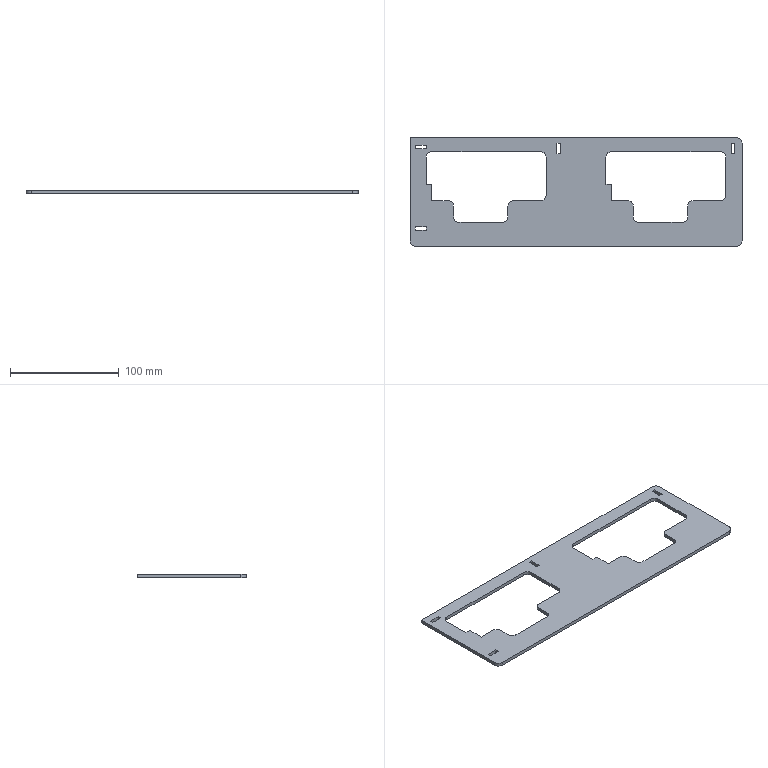Part | SolidWorks | features FlatPattern 1, SMBaseFlange 1, SheetMetal 1 | 1 solid | 59 faces | box 305 x 100 x 3.2 mm | volume 59642 mm3 | plane 42 | cylinder 17 | commonest cylinder face diameters 10 x17